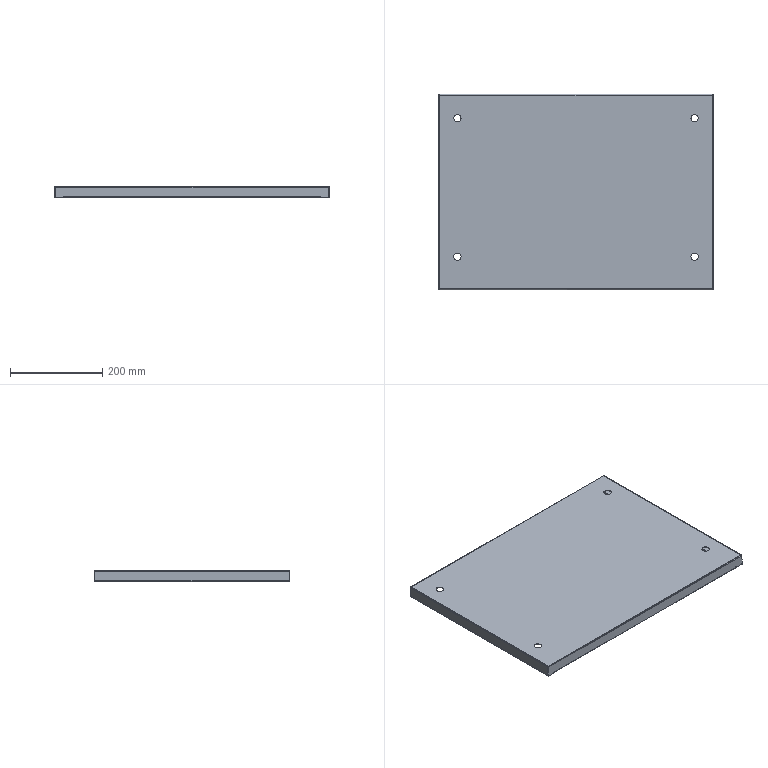Part | SolidWorks | features EdgeFlange 3, CornerFeat 1, Cut 1, FlatPattern 1, SMBaseFlange 1, SheetMetal 1 | 1 solid | 86 faces | box 593 x 423 x 25 mm | volume 482972 mm3 | plane 56 | cylinder 22 | spline 8 | commonest cylinder face diameters 16 x8 0.4 x7 3.4 x7